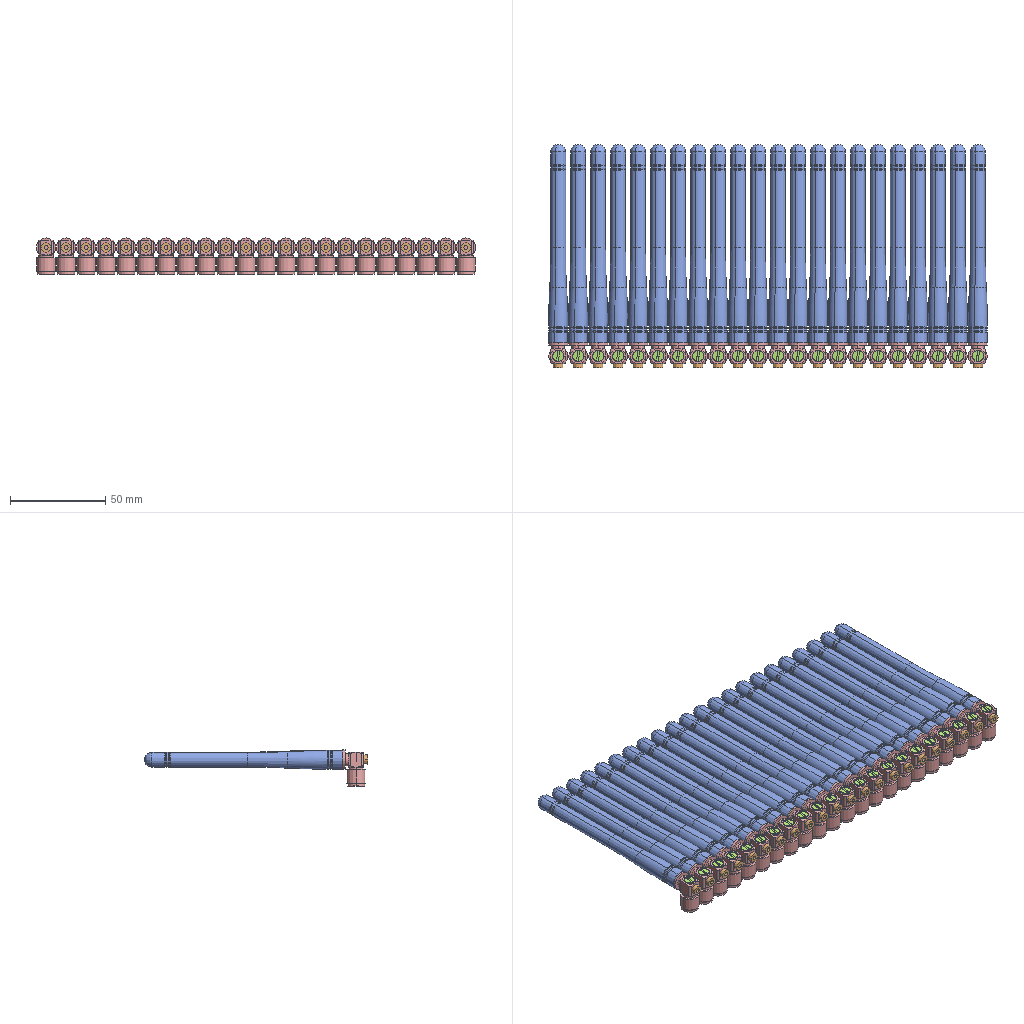Assembly | SolidWorks | 6 different items | 132 placed | box 231 x 117 x 19 mm
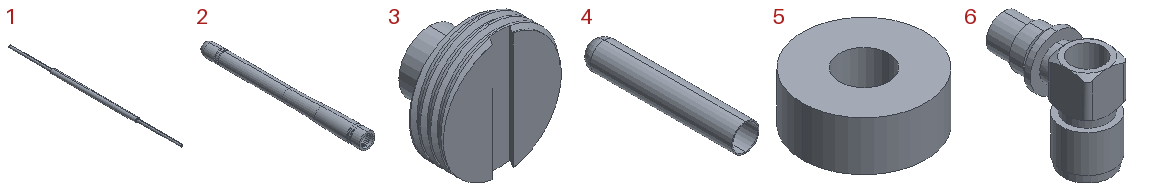Parts list (item | quantity | size | volume | features):
1 | x22 | 1.75 x 68.75 x 1.75 mm | 103.887 mm3 | features Revolution 1
2 | x22 | 10 x 104.2 x 10 mm | 2546 mm3 | features Fillet 1, Revolution 1
3 | x22 | 6 x 3.6 x 6 mm | 54.971 mm3 | features ICE 2, Extrusion 1, Helix 1, SweepCut 1
4 | x22 | 4.5 x 25.2 x 4.5 mm | 67.862 mm3 | features Revolution 1
5 | x22 | 5 x 5 x 2 mm | 32.987 mm3 | features Extrusion 1
6 | x22 | 10.2 x 20.95 x 19 mm | 1460 mm3 | features ICE 3, Revolution 2, Extrusion 1, Fillet 1, MirrorPattern 1, RevCut 1
Mates (type | each side: item.copy, entity, surface, feature):
Coordinate | 6.1 select_type:25 | assembly select_type:11
Concentric | 6.1 face cylinder Boss-Extrude2 | 2.1 face cylinder Revolve1
Coincident | 6.1 face plane Revolve1 | 2.1 face plane Revolve1
Concentric | 6.1 face cylinder Boss-Extrude2 | 1.1 face cylinder Revolve1
Concentric | 1.1 face cylinder Revolve1 | 4.1 face cylinder Revolve1
DistanceDim | 4.1 face plane Revolve1 | 6.1 face plane Boss-Extrude2
DistanceDim | 3.1 face plane Boss-Extrude1 | 6.1 face plane Boss-Extrude1
InPlace | 6.1 face plane Boss-Extrude1 | 5.1 plane